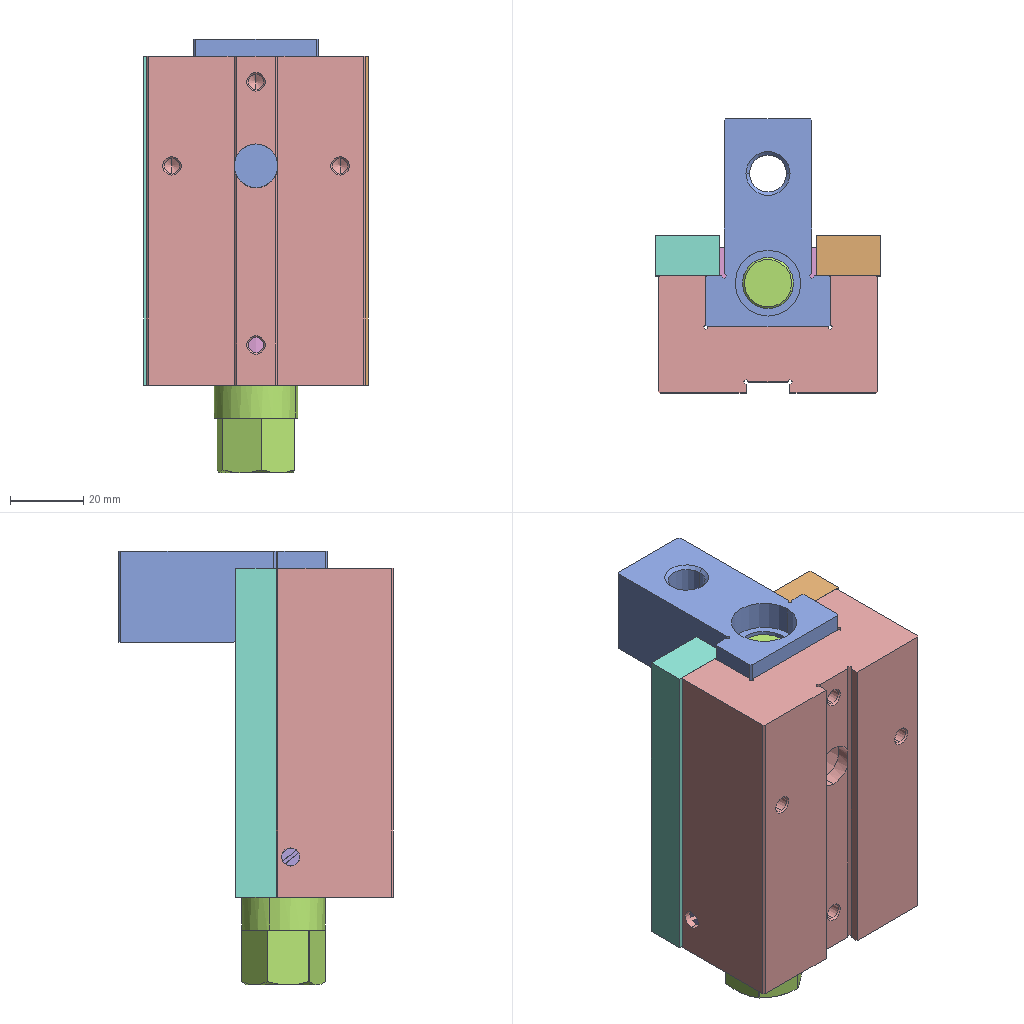Assembly | SolidWorks | 8 different items | 14 placed | box 61 x 75 x 119 mm
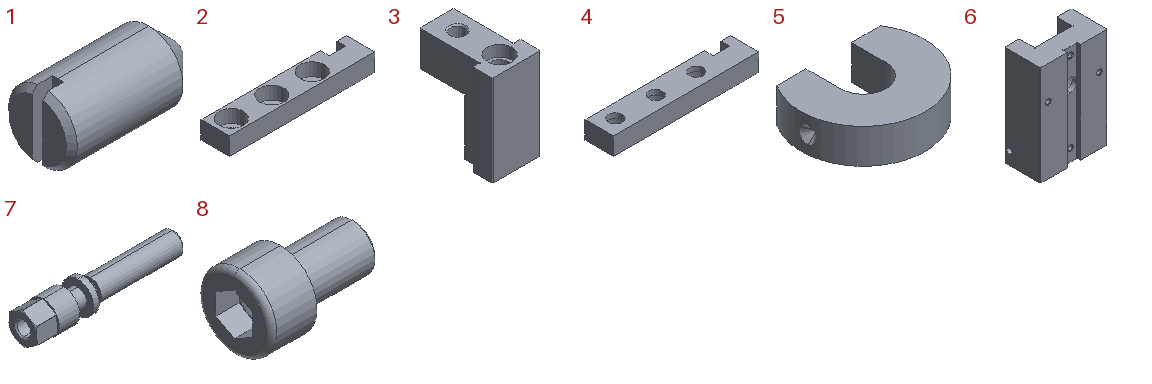Parts list (item | quantity | size | volume | features):
1 | x2 | 20 x 10 x 10 mm | 1349 mm3 | features Cut 1, LPattern 1, RevCut 1, Revolution 1
2 | x1 | 90 x 17.5 x 11 mm | 11956 mm3 | features Extrusion 1, ICE 1
3 | x1 | 34 x 57 x 65 mm | 53450 mm3 | features ICE 3, 3DProfileFeature 2, HoleWzd 2, Extrusion 1
4 | x1 | 90 x 17.5 x 11 mm | 11956 mm3 | features Extrusion 1, ICE 1
5 | x1 | 36 x 28 x 10 mm | 6463 mm3 | features Extrusion 1, MirrorPattern 1, RevCut 1
6 | x1 | 60 x 32 x 90 mm | 115385 mm3 | features 3DProfileFeature 4, HoleWzd 4, ICE 3, Extrusion 1
7 | x1 | 110 x 23 x 23 mm | 25098 mm3 | features 3DProfileFeature 1, Chamfer 1, HoleWzd 1, ICE 1, Revolution 1
8 | x6 | 26 x 16 x 16 mm | 2933 mm3 | features Fillet 2, RevCut 2, Boss 1, Chamfer 1, Cut 1, Extrusion 1, LPattern 1
Mates (type | each side: item.copy, entity, surface, feature):
Coincident | 6.1 face plane Boss-Extrude1 | 3.1 face plane Boss-Extrude1 | 2 times
Concentric | 3.1 face cylinder Cut-Extrude3 | 7.1 face cylinder Revolve1
Coincident | 6.1 face plane Cut-Extrude3 | 7.1 face plane Revolve1
Concentric | 6.1 face cylinder Cut-Extrude3 | 5.1 face cylinder Boss-Extrude1
Coincident | 6.1 face plane Cut-Extrude3 | 5.1 face plane Boss-Extrude1
Parallel | 6.1 face plane Boss-Extrude1 | 5.1 face plane Boss-Extrude1
Coincident | 6.1 face plane Boss-Extrude1 | 4.1 face plane Boss-Extrude1 | 2 times
Concentric | 6.1 face cylinder M8 Tapped Hole1 | 4.1 face cylinder Cut-Extrude1
Coincident | 6.1 face plane Boss-Extrude1 | 2.1 face plane Boss-Extrude1
Concentric | 6.1 face cylinder M8 Tapped Hole1 | 2.1 face cylinder Cut-Extrude1
Coincident | 4.1 face plane Boss-Extrude1 | 2.1 face plane Boss-Extrude1
Concentric | 6.1 face cylinder M6 Tapped Hole1 | 1.1 face cylinder Base
Concentric | 6.1 face cylinder M6 Tapped Hole1 | 1.2 face cylinder Base
Coincident | 5.1 face cone Cut-Revolve1 | 1.2 edge
Coincident | 5.1 face cone Mirror1 | 1.1 edge
Concentric | 2.1 face cylinder Cut-Extrude1 | 8.1 face cylinder BaseHead
Coincident | 2.1 face plane Cut-Extrude1 | 8.1 face plane BaseHead
Concentric | 2.1 face cylinder Cut-Extrude1 | 8.2 face cylinder BaseHead
Coincident | 2.1 face plane Cut-Extrude1 | 8.2 face plane BaseHead
Concentric | 2.1 face cylinder Cut-Extrude1 | 8.3 face cylinder BaseHead
Coincident | 2.1 face plane Cut-Extrude1 | 8.3 face plane BaseHead
Concentric | 4.1 face cylinder Cut-Extrude1 | 8.4 face cylinder BaseHead
Coincident | 4.1 face plane Cut-Extrude1 | 8.4 face plane BaseHead
Concentric | 4.1 face cylinder Cut-Extrude1 | 8.5 face cylinder BaseHead
Coincident | 4.1 face plane Cut-Extrude1 | 8.5 face plane BaseHead
Concentric | 4.1 face cylinder Cut-Extrude1 | 8.6 face cylinder BaseHead
Coincident | 4.1 face plane Cut-Extrude1 | 8.6 face plane BaseHead